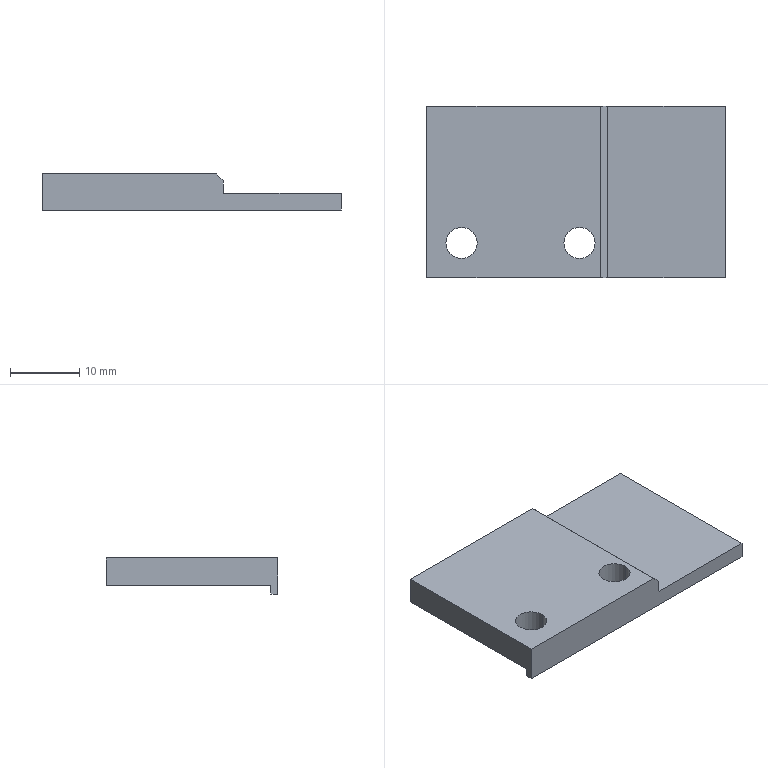Part | NX | 1 solid | 16 faces | box 43 x 24.7 x 5.2 mm | volume 2985 mm3 | plane 11 | cylinder 5 | commonest cylinder face diameters 4.5 x4 1 x1
STEP:
#1=CARTESIAN_POINT('',(0.,100.,-0.2));
#2=VERTEX_POINT('',#1);
#3=CARTESIAN_POINT('',(0.,101.,-0.2));
#4=VERTEX_POINT('',#3);
#5=CARTESIAN_POINT('',(0.,0.,-0.2));
#6=DIRECTION('',(0.,1.,0.));
#7=VECTOR('',#6,1000.);
#8=LINE('',#5,#7);
#9=EDGE_CURVE('',#2,#4,#8,.T.);
#10=ORIENTED_EDGE('',*,*,#9,.T.);
#11=CARTESIAN_POINT('',(43.,101.,-0.2));
#12=VERTEX_POINT('',#11);
#13=CARTESIAN_POINT('',(0.,101.,-0.2));
#14=DIRECTION('',(1.,0.,0.));
#15=VECTOR('',#14,1000.);
#16=LINE('',#13,#15);
#17=EDGE_CURVE('',#4,#12,#16,.T.);
#18=ORIENTED_EDGE('',*,*,#17,.T.);
#19=CARTESIAN_POINT('',(43.,100.,-0.2));
#20=VERTEX_POINT('',#19);
#21=CARTESIAN_POINT('',(43.,0.,-0.2));
#22=DIRECTION('',(0.,-1.,0.));
#23=VECTOR('',#22,1000.);
#24=LINE('',#21,#23);
#25=EDGE_CURVE('',#12,#20,#24,.T.);
#26=ORIENTED_EDGE('',*,*,#25,.T.);
#27=CARTESIAN_POINT('',(0.,100.,-0.2));
#28=DIRECTION('',(-1.,0.,0.));
#29=VECTOR('',#28,1000.);
#30=LINE('',#27,#29);
#31=EDGE_CURVE('',#20,#2,#30,.T.);
#32=ORIENTED_EDGE('',*,*,#31,.T.);
#33=EDGE_LOOP('',(#10,#18,#26,#32));
#34=FACE_BOUND('',#33,.T.);
#35=CARTESIAN_POINT('',(0.,100.,-0.2));
#36=DIRECTION('',(0.,0.,-1.));
#37=DIRECTION('',(0.,-1.,0.));
#38=AXIS2_PLACEMENT_3D('',#35,#36,#37);
#39=PLANE('',#38);
#40=ADVANCED_FACE('',(#34),#39,.T.);
#41=ORIENTED_EDGE('',*,*,#9,.F.);
#42=CARTESIAN_POINT('',(0.,100.,5.));
#43=VERTEX_POINT('',#42);
#44=CARTESIAN_POINT('',(0.,100.,0.));
#45=DIRECTION('',(0.,0.,1.));
#46=VECTOR('',#45,1000.);
#47=LINE('',#44,#46);
#48=EDGE_CURVE('',#2,#43,#47,.T.);
#49=ORIENTED_EDGE('',*,*,#48,.T.);
#50=CARTESIAN_POINT('',(0.,124.7,5.));
#51=VERTEX_POINT('',#50);
#52=CARTESIAN_POINT('',(0.,0.,5.));
#53=DIRECTION('',(0.,1.,0.));
#54=VECTOR('',#53,1000.);
#55=LINE('',#52,#54);
#56=EDGE_CURVE('',#43,#51,#55,.T.);
#57=ORIENTED_EDGE('',*,*,#56,.T.);
#58=CARTESIAN_POINT('',(0.,124.7,1.));
#59=VERTEX_POINT('',#58);
#60=CARTESIAN_POINT('',(0.,124.7,0.));
#61=DIRECTION('',(0.,0.,1.));
#62=VECTOR('',#61,1000.);
#63=LINE('',#60,#62);
#64=EDGE_CURVE('',#59,#51,#63,.T.);
#65=ORIENTED_EDGE('',*,*,#64,.F.);
#66=CARTESIAN_POINT('',(0.,101.,1.));
#67=VERTEX_POINT('',#66);
#68=CARTESIAN_POINT('',(0.,0.,1.));
#69=DIRECTION('',(0.,1.,0.));
#70=VECTOR('',#69,1000.);
#71=LINE('',#68,#70);
#72=EDGE_CURVE('',#67,#59,#71,.T.);
#73=ORIENTED_EDGE('',*,*,#72,.F.);
#74=CARTESIAN_POINT('',(0.,101.,0.));
#75=DIRECTION('',(0.,0.,1.));
#76=VECTOR('',#75,1000.);
#77=LINE('',#74,#76);
#78=EDGE_CURVE('',#4,#67,#77,.T.);
#79=ORIENTED_EDGE('',*,*,#78,.F.);
#80=EDGE_LOOP('',(#41,#49,#57,#65,#73,#79));
#81=FACE_BOUND('',#80,.T.);
#82=CARTESIAN_POINT('',(0.,100.,0.));
#83=DIRECTION('',(1.,0.,0.));
#84=DIRECTION('',(0.,1.,0.));
#85=AXIS2_PLACEMENT_3D('',#82,#83,#84);
#86=PLANE('',#85);
#87=ADVANCED_FACE('',(#81),#86,.F.);
#88=ORIENTED_EDGE('',*,*,#17,.F.);
#89=ORIENTED_EDGE('',*,*,#78,.T.);
#90=CARTESIAN_POINT('',(43.,101.,1.));
#91=VERTEX_POINT('',#90);
#92=CARTESIAN_POINT('',(0.,101.,1.));
#93=DIRECTION('',(-1.,0.,0.));
#94=VECTOR('',#93,1000.);
#95=LINE('',#92,#94);
#96=EDGE_CURVE('',#91,#67,#95,.T.);
#97=ORIENTED_EDGE('',*,*,#96,.F.);
#98=CARTESIAN_POINT('',(43.,101.,0.));
#99=DIRECTION('',(0.,0.,-1.));
#100=VECTOR('',#99,1000.);
#101=LINE('',#98,#100);
#102=EDGE_CURVE('',#91,#12,#101,.T.);
#103=ORIENTED_EDGE('',*,*,#102,.T.);
#104=EDGE_LOOP('',(#88,#89,#97,#103));
#105=FACE_BOUND('',#104,.T.);
#106=CARTESIAN_POINT('',(0.,101.,1.));
#107=DIRECTION('',(0.,1.,0.));
#108=DIRECTION('',(1.,0.,0.));
#109=AXIS2_PLACEMENT_3D('',#106,#107,#108);
#110=PLANE('',#109);
#111=ADVANCED_FACE('',(#105),#110,.T.);
#112=CARTESIAN_POINT('',(43.,100.,2.2));
#113=VERTEX_POINT('',#112);
#114=CARTESIAN_POINT('',(43.,124.7,2.2));
#115=VERTEX_POINT('',#114);
#116=CARTESIAN_POINT('',(43.,0.,2.2));
#117=DIRECTION('',(0.,1.,0.));
#118=VECTOR('',#117,1000.);
#119=LINE('',#116,#118);
#120=EDGE_CURVE('',#113,#115,#119,.T.);
#121=ORIENTED_EDGE('',*,*,#120,.F.);
#122=CARTESIAN_POINT('',(43.,100.,0.));
#123=DIRECTION('',(0.,0.,1.));
#124=VECTOR('',#123,1000.);
#125=LINE('',#122,#124);
#126=EDGE_CURVE('',#20,#113,#125,.T.);
#127=ORIENTED_EDGE('',*,*,#126,.F.);
#128=ORIENTED_EDGE('',*,*,#25,.F.);
#129=ORIENTED_EDGE('',*,*,#102,.F.);
#130=CARTESIAN_POINT('',(43.,124.7,1.));
#131=VERTEX_POINT('',#130);
#132=CARTESIAN_POINT('',(43.,0.,1.));
#133=DIRECTION('',(0.,-1.,0.));
#134=VECTOR('',#133,1000.);
#135=LINE('',#132,#134);
#136=EDGE_CURVE('',#131,#91,#135,.T.);
#137=ORIENTED_EDGE('',*,*,#136,.F.);
#138=CARTESIAN_POINT('',(43.,124.7,0.));
#139=DIRECTION('',(0.,0.,-1.));
#140=VECTOR('',#139,1000.);
#141=LINE('',#138,#140);
#142=EDGE_CURVE('',#115,#131,#141,.T.);
#143=ORIENTED_EDGE('',*,*,#142,.F.);
#144=EDGE_LOOP('',(#121,#127,#128,#129,#137,#143));
#145=FACE_BOUND('',#144,.T.);
#146=CARTESIAN_POINT('',(43.,126.7,0.));
#147=DIRECTION('',(-1.,0.,0.));
#148=DIRECTION('',(0.,0.,1.));
#149=AXIS2_PLACEMENT_3D('',#146,#147,#148);
#150=PLANE('',#149);
#151=ADVANCED_FACE('',(#145),#150,.F.);
#152=CARTESIAN_POINT('',(26.1,100.,2.2));
#153=VERTEX_POINT('',#152);
#154=CARTESIAN_POINT('',(26.1,124.7,2.2));
#155=VERTEX_POINT('',#154);
#156=CARTESIAN_POINT('',(26.1,126.782,2.2));
#157=DIRECTION('',(0.,1.,0.));
#158=VECTOR('',#157,1000.);
#159=LINE('',#156,#158);
#160=EDGE_CURVE('',#153,#155,#159,.T.);
#161=ORIENTED_EDGE('',*,*,#160,.F.);
#162=CARTESIAN_POINT('',(0.,100.,2.2));
#163=DIRECTION('',(1.,0.,0.));
#164=VECTOR('',#163,1000.);
#165=LINE('',#162,#164);
#166=EDGE_CURVE('',#153,#113,#165,.T.);
#167=ORIENTED_EDGE('',*,*,#166,.T.);
#168=ORIENTED_EDGE('',*,*,#120,.T.);
#169=CARTESIAN_POINT('',(0.,124.7,2.2));
#170=DIRECTION('',(-1.,0.,0.));
#171=VECTOR('',#170,1000.);
#172=LINE('',#169,#171);
#173=EDGE_CURVE('',#115,#155,#172,.T.);
#174=ORIENTED_EDGE('',*,*,#173,.T.);
#175=EDGE_LOOP('',(#161,#167,#168,#174));
#176=FACE_BOUND('',#175,.T.);
#177=CARTESIAN_POINT('',(0.,100.,2.2));
#178=DIRECTION('',(0.,0.,-1.));
#179=DIRECTION('',(0.,-1.,0.));
#180=AXIS2_PLACEMENT_3D('',#177,#178,#179);
#181=PLANE('',#180);
#182=ADVANCED_FACE('',(#176),#181,.F.);
#183=ORIENTED_EDGE('',*,*,#160,.T.);
#184=CARTESIAN_POINT('',(26.,124.7,2.5));
#185=VERTEX_POINT('',#184);
#186=CARTESIAN_POINT('',(26.5,124.7,2.5));
#187=DIRECTION('',(0.,1.,0.));
#188=DIRECTION('',(0.,0.,-1.));
#189=AXIS2_PLACEMENT_3D('',#186,#187,#188);
#190=CIRCLE('',#189,0.5);
#191=EDGE_CURVE('',#155,#185,#190,.T.);
#192=ORIENTED_EDGE('',*,*,#191,.T.);
#193=CARTESIAN_POINT('',(26.,100.,2.5));
#194=VERTEX_POINT('',#193);
#195=CARTESIAN_POINT('',(26.,100.,2.5));
#196=DIRECTION('',(0.,1.,0.));
#197=VECTOR('',#196,1000.);
#198=LINE('',#195,#197);
#199=EDGE_CURVE('',#194,#185,#198,.T.);
#200=ORIENTED_EDGE('',*,*,#199,.F.);
#201=CARTESIAN_POINT('',(26.5,100.,2.5));
#202=DIRECTION('',(0.,1.,0.));
#203=DIRECTION('',(0.,0.,-1.));
#204=AXIS2_PLACEMENT_3D('',#201,#202,#203);
#205=CIRCLE('',#204,0.5);
#206=EDGE_CURVE('',#153,#194,#205,.T.);
#207=ORIENTED_EDGE('',*,*,#206,.F.);
#208=EDGE_LOOP('',(#183,#192,#200,#207));
#209=FACE_BOUND('',#208,.T.);
#210=CARTESIAN_POINT('',(26.5,126.782,2.5));
#211=DIRECTION('',(0.,1.,0.));
#212=DIRECTION('',(0.,0.,-1.));
#213=AXIS2_PLACEMENT_3D('',#210,#211,#212);
#214=CYLINDRICAL_SURFACE('',#213,0.5);
#215=ADVANCED_FACE('',(#209),#214,.F.);
#216=ORIENTED_EDGE('',*,*,#166,.F.);
#217=ORIENTED_EDGE('',*,*,#206,.T.);
#218=CARTESIAN_POINT('',(26.,100.,4.));
#219=VERTEX_POINT('',#218);
#220=CARTESIAN_POINT('',(26.,100.,0.));
#221=DIRECTION('',(0.,0.,1.));
#222=VECTOR('',#221,1000.);
#223=LINE('',#220,#222);
#224=EDGE_CURVE('',#194,#219,#223,.T.);
#225=ORIENTED_EDGE('',*,*,#224,.T.);
#226=CARTESIAN_POINT('',(25.,100.,5.));
#227=VERTEX_POINT('',#226);
#228=CARTESIAN_POINT('',(30.,100.,0.));
#229=DIRECTION('',(-0.7071,0.,0.7071));
#230=VECTOR('',#229,1000.);
#231=LINE('',#228,#230);
#232=EDGE_CURVE('',#219,#227,#231,.T.);
#233=ORIENTED_EDGE('',*,*,#232,.T.);
#234=CARTESIAN_POINT('',(0.,100.,5.));
#235=DIRECTION('',(-1.,0.,0.));
#236=VECTOR('',#235,1000.);
#237=LINE('',#234,#236);
#238=EDGE_CURVE('',#227,#43,#237,.T.);
#239=ORIENTED_EDGE('',*,*,#238,.T.);
#240=ORIENTED_EDGE('',*,*,#48,.F.);
#241=ORIENTED_EDGE('',*,*,#31,.F.);
#242=ORIENTED_EDGE('',*,*,#126,.T.);
#243=EDGE_LOOP('',(#216,#217,#225,#233,#239,#240,#241,#242));
#244=FACE_BOUND('',#243,.T.);
#245=CARTESIAN_POINT('',(43.,100.,0.));
#246=DIRECTION('',(0.,1.,0.));
#247=DIRECTION('',(1.,0.,0.));
#248=AXIS2_PLACEMENT_3D('',#245,#246,#247);
#249=PLANE('',#248);
#250=ADVANCED_FACE('',(#244),#249,.F.);
#251=CARTESIAN_POINT('',(25.,124.7,5.));
#252=VERTEX_POINT('',#251);
#253=CARTESIAN_POINT('',(25.,0.,5.));
#254=DIRECTION('',(0.,1.,0.));
#255=VECTOR('',#254,1000.);
#256=LINE('',#253,#255);
#257=EDGE_CURVE('',#227,#252,#256,.T.);
#258=ORIENTED_EDGE('',*,*,#257,.T.);
#259=CARTESIAN_POINT('',(0.,124.7,5.));
#260=DIRECTION('',(1.,0.,0.));
#261=VECTOR('',#260,1000.);
#262=LINE('',#259,#261);
#263=EDGE_CURVE('',#51,#252,#262,.T.);
#264=ORIENTED_EDGE('',*,*,#263,.F.);
#265=ORIENTED_EDGE('',*,*,#56,.F.);
#266=ORIENTED_EDGE('',*,*,#238,.F.);
#267=EDGE_LOOP('',(#258,#264,#265,#266));
#268=FACE_BOUND('',#267,.T.);
#269=CARTESIAN_POINT('',(24.25,105.,5.));
#270=VERTEX_POINT('',#269);
#271=CARTESIAN_POINT('',(19.75,105.,5.));
#272=VERTEX_POINT('',#271);
#273=CARTESIAN_POINT('',(22.,105.,5.));
#274=DIRECTION('',(0.,0.,1.));
#275=DIRECTION('',(-1.,0.,0.));
#276=AXIS2_PLACEMENT_3D('',#273,#274,#275);
#277=CIRCLE('',#276,2.25);
#278=EDGE_CURVE('',#270,#272,#277,.T.);
#279=ORIENTED_EDGE('',*,*,#278,.F.);
#280=CARTESIAN_POINT('',(22.,105.,5.));
#281=DIRECTION('',(0.,0.,1.));
#282=DIRECTION('',(-1.,0.,0.));
#283=AXIS2_PLACEMENT_3D('',#280,#281,#282);
#284=CIRCLE('',#283,2.25);
#285=EDGE_CURVE('',#272,#270,#284,.T.);
#286=ORIENTED_EDGE('',*,*,#285,.F.);
#287=EDGE_LOOP('',(#279,#286));
#288=FACE_BOUND('',#287,.T.);
#289=CARTESIAN_POINT('',(7.25,105.,5.));
#290=VERTEX_POINT('',#289);
#291=CARTESIAN_POINT('',(2.75,105.,5.));
#292=VERTEX_POINT('',#291);
#293=CARTESIAN_POINT('',(5.,105.,5.));
#294=DIRECTION('',(0.,0.,1.));
#295=DIRECTION('',(-1.,0.,0.));
#296=AXIS2_PLACEMENT_3D('',#293,#294,#295);
#297=CIRCLE('',#296,2.25);
#298=EDGE_CURVE('',#290,#292,#297,.T.);
#299=ORIENTED_EDGE('',*,*,#298,.F.);
#300=CARTESIAN_POINT('',(5.,105.,5.));
#301=DIRECTION('',(0.,0.,1.));
#302=DIRECTION('',(-1.,0.,0.));
#303=AXIS2_PLACEMENT_3D('',#300,#301,#302);
#304=CIRCLE('',#303,2.25);
#305=EDGE_CURVE('',#292,#290,#304,.T.);
#306=ORIENTED_EDGE('',*,*,#305,.F.);
#307=EDGE_LOOP('',(#299,#306));
#308=FACE_BOUND('',#307,.T.);
#309=CARTESIAN_POINT('',(0.,100.,5.));
#310=DIRECTION('',(0.,0.,-1.));
#311=DIRECTION('',(0.,-1.,0.));
#312=AXIS2_PLACEMENT_3D('',#309,#310,#311);
#313=PLANE('',#312);
#314=ADVANCED_FACE('',(#268,#288,#308),#313,.F.);
#315=ORIENTED_EDGE('',*,*,#199,.T.);
#316=CARTESIAN_POINT('',(26.,124.7,4.));
#317=VERTEX_POINT('',#316);
#318=CARTESIAN_POINT('',(26.,124.7,0.));
#319=DIRECTION('',(0.,0.,-1.));
#320=VECTOR('',#319,1000.);
#321=LINE('',#318,#320);
#322=EDGE_CURVE('',#317,#185,#321,.T.);
#323=ORIENTED_EDGE('',*,*,#322,.F.);
#324=CARTESIAN_POINT('',(26.,0.,4.));
#325=DIRECTION('',(0.,-1.,0.));
#326=VECTOR('',#325,1000.);
#327=LINE('',#324,#326);
#328=EDGE_CURVE('',#317,#219,#327,.T.);
#329=ORIENTED_EDGE('',*,*,#328,.T.);
#330=ORIENTED_EDGE('',*,*,#224,.F.);
#331=EDGE_LOOP('',(#315,#323,#329,#330));
#332=FACE_BOUND('',#331,.T.);
#333=CARTESIAN_POINT('',(26.,100.,5.));
#334=DIRECTION('',(1.,0.,0.));
#335=DIRECTION('',(0.,1.,0.));
#336=AXIS2_PLACEMENT_3D('',#333,#334,#335);
#337=PLANE('',#336);
#338=ADVANCED_FACE('',(#332),#337,.T.);
#339=ORIENTED_EDGE('',*,*,#322,.T.);
#340=ORIENTED_EDGE('',*,*,#191,.F.);
#341=ORIENTED_EDGE('',*,*,#173,.F.);
#342=ORIENTED_EDGE('',*,*,#142,.T.);
#343=CARTESIAN_POINT('',(0.,124.7,1.));
#344=DIRECTION('',(1.,0.,0.));
#345=VECTOR('',#344,1000.);
#346=LINE('',#343,#345);
#347=EDGE_CURVE('',#59,#131,#346,.T.);
#348=ORIENTED_EDGE('',*,*,#347,.F.);
#349=ORIENTED_EDGE('',*,*,#64,.T.);
#350=ORIENTED_EDGE('',*,*,#263,.T.);
#351=CARTESIAN_POINT('',(30.,124.7,0.));
#352=DIRECTION('',(0.7071,0.,-0.7071));
#353=VECTOR('',#352,1000.);
#354=LINE('',#351,#353);
#355=EDGE_CURVE('',#252,#317,#354,.T.);
#356=ORIENTED_EDGE('',*,*,#355,.T.);
#357=EDGE_LOOP('',(#339,#340,#341,#342,#348,#349,#350,#356));
#358=FACE_BOUND('',#357,.T.);
#359=CARTESIAN_POINT('',(0.,124.7,0.));
#360=DIRECTION('',(0.,-1.,0.));
#361=DIRECTION('',(0.,0.,-1.));
#362=AXIS2_PLACEMENT_3D('',#359,#360,#361);
#363=PLANE('',#362);
#364=ADVANCED_FACE('',(#358),#363,.F.);
#365=ORIENTED_EDGE('',*,*,#72,.T.);
#366=ORIENTED_EDGE('',*,*,#347,.T.);
#367=ORIENTED_EDGE('',*,*,#136,.T.);
#368=ORIENTED_EDGE('',*,*,#96,.T.);
#369=EDGE_LOOP('',(#365,#366,#367,#368));
#370=FACE_BOUND('',#369,.T.);
#371=CARTESIAN_POINT('',(19.75,105.,1.));
#372=VERTEX_POINT('',#371);
#373=CARTESIAN_POINT('',(24.25,105.,1.));
#374=VERTEX_POINT('',#373);
#375=CARTESIAN_POINT('',(22.,105.,1.));
#376=DIRECTION('',(0.,0.,1.));
#377=DIRECTION('',(-1.,0.,0.));
#378=AXIS2_PLACEMENT_3D('',#375,#376,#377);
#379=CIRCLE('',#378,2.25);
#380=EDGE_CURVE('',#372,#374,#379,.T.);
#381=ORIENTED_EDGE('',*,*,#380,.T.);
#382=CARTESIAN_POINT('',(22.,105.,1.));
#383=DIRECTION('',(0.,0.,1.));
#384=DIRECTION('',(-1.,0.,0.));
#385=AXIS2_PLACEMENT_3D('',#382,#383,#384);
#386=CIRCLE('',#385,2.25);
#387=EDGE_CURVE('',#374,#372,#386,.T.);
#388=ORIENTED_EDGE('',*,*,#387,.T.);
#389=EDGE_LOOP('',(#381,#388));
#390=FACE_BOUND('',#389,.T.);
#391=CARTESIAN_POINT('',(2.75,105.,1.));
#392=VERTEX_POINT('',#391);
#393=CARTESIAN_POINT('',(7.25,105.,1.));
#394=VERTEX_POINT('',#393);
#395=CARTESIAN_POINT('',(5.,105.,1.));
#396=DIRECTION('',(0.,0.,1.));
#397=DIRECTION('',(-1.,0.,0.));
#398=AXIS2_PLACEMENT_3D('',#395,#396,#397);
#399=CIRCLE('',#398,2.25);
#400=EDGE_CURVE('',#392,#394,#399,.T.);
#401=ORIENTED_EDGE('',*,*,#400,.T.);
#402=CARTESIAN_POINT('',(5.,105.,1.));
#403=DIRECTION('',(0.,0.,1.));
#404=DIRECTION('',(-1.,0.,0.));
#405=AXIS2_PLACEMENT_3D('',#402,#403,#404);
#406=CIRCLE('',#405,2.25);
#407=EDGE_CURVE('',#394,#392,#406,.T.);
#408=ORIENTED_EDGE('',*,*,#407,.T.);
#409=EDGE_LOOP('',(#401,#408));
#410=FACE_BOUND('',#409,.T.);
#411=CARTESIAN_POINT('',(0.,126.7,1.));
#412=DIRECTION('',(0.,0.,-1.));
#413=DIRECTION('',(0.,-1.,0.));
#414=AXIS2_PLACEMENT_3D('',#411,#412,#413);
#415=PLANE('',#414);
#416=ADVANCED_FACE('',(#370,#390,#410),#415,.T.);
#417=ORIENTED_EDGE('',*,*,#278,.T.);
#418=CARTESIAN_POINT('',(19.75,105.,5.));
#419=DIRECTION('',(0.,0.,1.));
#420=VECTOR('',#419,1000.);
#421=LINE('',#418,#420);
#422=EDGE_CURVE('',#272,#372,#421,.F.);
#423=ORIENTED_EDGE('',*,*,#422,.T.);
#424=ORIENTED_EDGE('',*,*,#387,.F.);
#425=CARTESIAN_POINT('',(24.25,105.,5.));
#426=DIRECTION('',(0.,0.,1.));
#427=VECTOR('',#426,1000.);
#428=LINE('',#425,#427);
#429=EDGE_CURVE('',#270,#374,#428,.F.);
#430=ORIENTED_EDGE('',*,*,#429,.F.);
#431=EDGE_LOOP('',(#417,#423,#424,#430));
#432=FACE_BOUND('',#431,.T.);
#433=CARTESIAN_POINT('',(22.,105.,5.));
#434=DIRECTION('',(0.,0.,1.));
#435=DIRECTION('',(-1.,0.,0.));
#436=AXIS2_PLACEMENT_3D('',#433,#434,#435);
#437=CYLINDRICAL_SURFACE('',#436,2.25);
#438=ADVANCED_FACE('',(#432),#437,.F.);
#439=ORIENTED_EDGE('',*,*,#400,.F.);
#440=CARTESIAN_POINT('',(2.75,105.,5.));
#441=DIRECTION('',(0.,0.,1.));
#442=VECTOR('',#441,1000.);
#443=LINE('',#440,#442);
#444=EDGE_CURVE('',#292,#392,#443,.F.);
#445=ORIENTED_EDGE('',*,*,#444,.F.);
#446=ORIENTED_EDGE('',*,*,#305,.T.);
#447=CARTESIAN_POINT('',(7.25,105.,5.));
#448=DIRECTION('',(0.,0.,1.));
#449=VECTOR('',#448,1000.);
#450=LINE('',#447,#449);
#451=EDGE_CURVE('',#290,#394,#450,.F.);
#452=ORIENTED_EDGE('',*,*,#451,.T.);
#453=EDGE_LOOP('',(#439,#445,#446,#452));
#454=FACE_BOUND('',#453,.T.);
#455=CARTESIAN_POINT('',(5.,105.,5.));
#456=DIRECTION('',(0.,0.,1.));
#457=DIRECTION('',(-1.,0.,0.));
#458=AXIS2_PLACEMENT_3D('',#455,#456,#457);
#459=CYLINDRICAL_SURFACE('',#458,2.25);
#460=ADVANCED_FACE('',(#454),#459,.F.);
#461=ORIENTED_EDGE('',*,*,#257,.F.);
#462=ORIENTED_EDGE('',*,*,#232,.F.);
#463=ORIENTED_EDGE('',*,*,#328,.F.);
#464=ORIENTED_EDGE('',*,*,#355,.F.);
#465=EDGE_LOOP('',(#461,#462,#463,#464));
#466=FACE_BOUND('',#465,.T.);
#467=CARTESIAN_POINT('',(25.5,113.35,4.5));
#468=DIRECTION('',(0.7071,0.,0.7071));
#469=DIRECTION('',(0.,-1.,0.));
#470=AXIS2_PLACEMENT_3D('',#467,#468,#469);
#471=PLANE('',#470);
#472=ADVANCED_FACE('',(#466),#471,.T.);
#473=ORIENTED_EDGE('',*,*,#380,.F.);
#474=ORIENTED_EDGE('',*,*,#422,.F.);
#475=ORIENTED_EDGE('',*,*,#285,.T.);
#476=ORIENTED_EDGE('',*,*,#429,.T.);
#477=EDGE_LOOP('',(#473,#474,#475,#476));
#478=FACE_BOUND('',#477,.T.);
#479=CARTESIAN_POINT('',(22.,105.,5.));
#480=DIRECTION('',(0.,0.,1.));
#481=DIRECTION('',(-1.,0.,0.));
#482=AXIS2_PLACEMENT_3D('',#479,#480,#481);
#483=CYLINDRICAL_SURFACE('',#482,2.25);
#484=ADVANCED_FACE('',(#478),#483,.F.);
#485=ORIENTED_EDGE('',*,*,#298,.T.);
#486=ORIENTED_EDGE('',*,*,#444,.T.);
#487=ORIENTED_EDGE('',*,*,#407,.F.);
#488=ORIENTED_EDGE('',*,*,#451,.F.);
#489=EDGE_LOOP('',(#485,#486,#487,#488));
#490=FACE_BOUND('',#489,.T.);
#491=CARTESIAN_POINT('',(5.,105.,5.));
#492=DIRECTION('',(0.,0.,1.));
#493=DIRECTION('',(-1.,0.,0.));
#494=AXIS2_PLACEMENT_3D('',#491,#492,#493);
#495=CYLINDRICAL_SURFACE('',#494,2.25);
#496=ADVANCED_FACE('',(#490),#495,.F.);
#497=CLOSED_SHELL('',(#40,#87,#111,#151,#182,#215,#250,#314,#338,#364,#416,#438,#460,#472,#484,#496));
#498=MANIFOLD_SOLID_BREP('',#497);
#499=(LENGTH_UNIT()NAMED_UNIT(*)SI_UNIT(.MILLI.,.METRE.));
#500=UNCERTAINTY_MEASURE_WITH_UNIT(LENGTH_MEASURE(0.00001),#499,'','');
#501=(NAMED_UNIT(*)PLANE_ANGLE_UNIT()SI_UNIT($,.RADIAN.));
#502=(NAMED_UNIT(*)SI_UNIT($,.STERADIAN.)SOLID_ANGLE_UNIT());
#503=(GEOMETRIC_REPRESENTATION_CONTEXT(3)GLOBAL_UNCERTAINTY_ASSIGNED_CONTEXT((#500))GLOBAL_UNIT_ASSIGNED_CONTEXT((#499,#501,#502))REPRESENTATION_CONTEXT('',''));
#504=ADVANCED_BREP_SHAPE_REPRESENTATION('',(#498),#503);